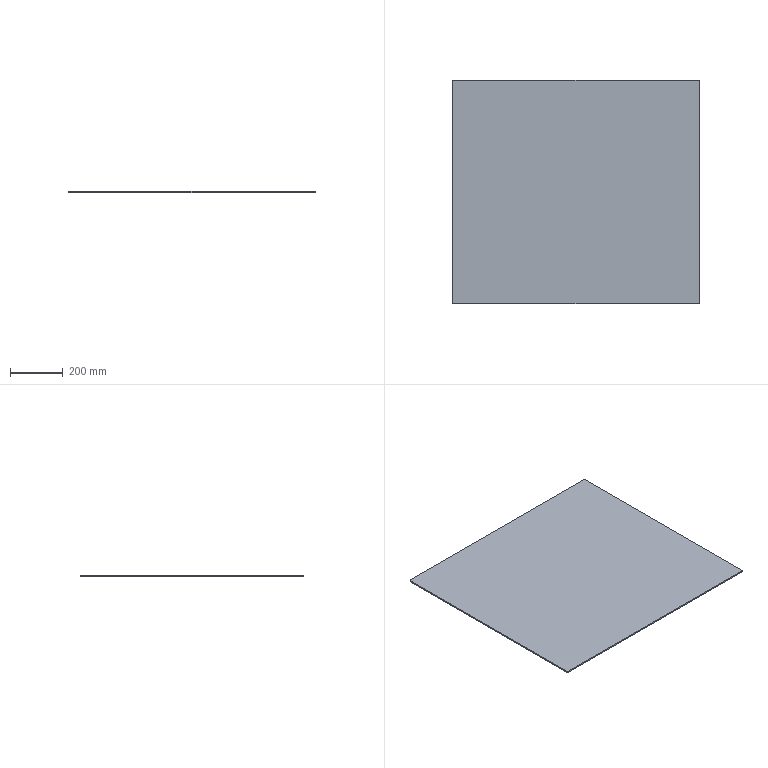Part | STEP file | 001-002-Face Plate-8 | 1 solid | 10 faces | box 940 x 850 x 5 mm | volume 3994893 mm3 | plane 6 | cylinder 4 | commonest cylinder face diameters 10 x4
STEP:
#1=CARTESIAN_POINT('',(0.,0.,0.));
#2=DIRECTION('',(0.,0.,1.));
#3=DIRECTION('',(1.,0.,0.));
#4=AXIS2_PLACEMENT_3D('',#1,#2,#3);
#5=CARTESIAN_POINT('',(470.,-420.,0.));
#6=VERTEX_POINT('',#5);
#7=CARTESIAN_POINT('',(470.,420.,0.));
#8=VERTEX_POINT('',#7);
#9=CARTESIAN_POINT('',(470.,-425.,0.));
#10=DIRECTION('',(0.,1.,0.));
#11=VECTOR('',#10,1.);
#12=LINE('',#9,#11);
#13=CARTESIAN_POINT('',(470.,-425.,5.));
#14=DIRECTION('',(-1.,0.,0.));
#15=DIRECTION('',(0.,0.,1.));
#16=AXIS2_PLACEMENT_3D('',#13,#14,#15);
#17=PLANE('',#16);
#18=CARTESIAN_POINT('',(-5.,0.));
#19=DIRECTION('',(0.,1.));
#20=VECTOR('',#19,1.);
#21=LINE('',#18,#20);
#22=(GEOMETRIC_REPRESENTATION_CONTEXT(2)PARAMETRIC_REPRESENTATION_CONTEXT()REPRESENTATION_CONTEXT('',''));
#23=DEFINITIONAL_REPRESENTATION('',(#21),#22);
#24=PCURVE('',#17,#23);
#25=CARTESIAN_POINT('',(0.,0.,0.));
#26=DIRECTION('',(0.,0.,-1.));
#27=DIRECTION('',(-1.,0.,0.));
#28=AXIS2_PLACEMENT_3D('',#25,#26,#27);
#29=PLANE('',#28);
#30=CARTESIAN_POINT('',(-470.,-425.));
#31=DIRECTION('',(0.,1.));
#32=VECTOR('',#31,1.);
#33=LINE('',#30,#32);
#34=(GEOMETRIC_REPRESENTATION_CONTEXT(2)PARAMETRIC_REPRESENTATION_CONTEXT()REPRESENTATION_CONTEXT('',''));
#35=DEFINITIONAL_REPRESENTATION('',(#33),#34);
#36=PCURVE('',#29,#35);
#37=SURFACE_CURVE('',#12,(#24,#36),.PCURVE_S1.);
#38=EDGE_CURVE('',#6,#8,#37,.T.);
#39=ORIENTED_EDGE('',*,*,#38,.T.);
#40=CARTESIAN_POINT('',(470.,420.,5.));
#41=VERTEX_POINT('',#40);
#42=CARTESIAN_POINT('',(470.,420.,5.));
#43=DIRECTION('',(0.,0.,1.));
#44=VECTOR('',#43,1.);
#45=LINE('',#42,#44);
#46=CARTESIAN_POINT('',(0.,845.));
#47=DIRECTION('',(1.,0.));
#48=VECTOR('',#47,1.);
#49=LINE('',#46,#48);
#50=(GEOMETRIC_REPRESENTATION_CONTEXT(2)PARAMETRIC_REPRESENTATION_CONTEXT()REPRESENTATION_CONTEXT('',''));
#51=DEFINITIONAL_REPRESENTATION('',(#49),#50);
#52=PCURVE('',#17,#51);
#53=CARTESIAN_POINT('',(465.,420.,5.));
#54=DIRECTION('',(0.,0.,-1.));
#55=DIRECTION('',(-1.,0.,0.));
#56=AXIS2_PLACEMENT_3D('',#53,#54,#55);
#57=CYLINDRICAL_SURFACE('',#56,5.);
#58=CARTESIAN_POINT('',(3.142,0.));
#59=DIRECTION('',(0.,-1.));
#60=VECTOR('',#59,1.);
#61=LINE('',#58,#60);
#62=(GEOMETRIC_REPRESENTATION_CONTEXT(2)PARAMETRIC_REPRESENTATION_CONTEXT()REPRESENTATION_CONTEXT('',''));
#63=DEFINITIONAL_REPRESENTATION('',(#61),#62);
#64=PCURVE('',#57,#63);
#65=SURFACE_CURVE('',#45,(#52,#64),.PCURVE_S1.);
#66=EDGE_CURVE('',#8,#41,#65,.T.);
#67=ORIENTED_EDGE('',*,*,#66,.T.);
#68=CARTESIAN_POINT('',(470.,-420.,5.));
#69=VERTEX_POINT('',#68);
#70=CARTESIAN_POINT('',(470.,-425.,5.));
#71=DIRECTION('',(0.,1.,0.));
#72=VECTOR('',#71,1.);
#73=LINE('',#70,#72);
#74=CARTESIAN_POINT('',(0.,0.));
#75=DIRECTION('',(0.,1.));
#76=VECTOR('',#75,1.);
#77=LINE('',#74,#76);
#78=(GEOMETRIC_REPRESENTATION_CONTEXT(2)PARAMETRIC_REPRESENTATION_CONTEXT()REPRESENTATION_CONTEXT('',''));
#79=DEFINITIONAL_REPRESENTATION('',(#77),#78);
#80=PCURVE('',#17,#79);
#81=CARTESIAN_POINT('',(0.,0.,5.));
#82=DIRECTION('',(0.,0.,-1.));
#83=DIRECTION('',(-1.,0.,0.));
#84=AXIS2_PLACEMENT_3D('',#81,#82,#83);
#85=PLANE('',#84);
#86=CARTESIAN_POINT('',(-470.,-425.));
#87=DIRECTION('',(0.,1.));
#88=VECTOR('',#87,1.);
#89=LINE('',#86,#88);
#90=(GEOMETRIC_REPRESENTATION_CONTEXT(2)PARAMETRIC_REPRESENTATION_CONTEXT()REPRESENTATION_CONTEXT('',''));
#91=DEFINITIONAL_REPRESENTATION('',(#89),#90);
#92=PCURVE('',#85,#91);
#93=SURFACE_CURVE('',#73,(#80,#92),.PCURVE_S1.);
#94=EDGE_CURVE('',#69,#41,#93,.T.);
#95=ORIENTED_EDGE('',*,*,#94,.F.);
#96=CARTESIAN_POINT('',(470.,-420.,5.));
#97=DIRECTION('',(0.,0.,-1.));
#98=VECTOR('',#97,1.);
#99=LINE('',#96,#98);
#100=CARTESIAN_POINT('',(0.,5.));
#101=DIRECTION('',(-1.,0.));
#102=VECTOR('',#101,1.);
#103=LINE('',#100,#102);
#104=(GEOMETRIC_REPRESENTATION_CONTEXT(2)PARAMETRIC_REPRESENTATION_CONTEXT()REPRESENTATION_CONTEXT('',''));
#105=DEFINITIONAL_REPRESENTATION('',(#103),#104);
#106=PCURVE('',#17,#105);
#107=CARTESIAN_POINT('',(465.,-420.,5.));
#108=DIRECTION('',(0.,0.,-1.));
#109=DIRECTION('',(-1.,0.,0.));
#110=AXIS2_PLACEMENT_3D('',#107,#108,#109);
#111=CYLINDRICAL_SURFACE('',#110,5.);
#112=CARTESIAN_POINT('',(3.142,0.));
#113=DIRECTION('',(0.,1.));
#114=VECTOR('',#113,1.);
#115=LINE('',#112,#114);
#116=(GEOMETRIC_REPRESENTATION_CONTEXT(2)PARAMETRIC_REPRESENTATION_CONTEXT()REPRESENTATION_CONTEXT('',''));
#117=DEFINITIONAL_REPRESENTATION('',(#115),#116);
#118=PCURVE('',#111,#117);
#119=SURFACE_CURVE('',#99,(#106,#118),.PCURVE_S1.);
#120=EDGE_CURVE('',#69,#6,#119,.T.);
#121=ORIENTED_EDGE('',*,*,#120,.T.);
#122=EDGE_LOOP('',(#39,#67,#95,#121));
#123=FACE_BOUND('',#122,.T.);
#124=ADVANCED_FACE('',(#123),#17,.F.);
#125=CARTESIAN_POINT('',(465.,425.,0.));
#126=VERTEX_POINT('',#125);
#127=CARTESIAN_POINT('',(-465.,425.,0.));
#128=VERTEX_POINT('',#127);
#129=CARTESIAN_POINT('',(-470.,425.,0.));
#130=DIRECTION('',(-1.,0.,0.));
#131=VECTOR('',#130,1.);
#132=LINE('',#129,#131);
#133=CARTESIAN_POINT('',(-470.,425.,5.));
#134=DIRECTION('',(0.,-1.,0.));
#135=DIRECTION('',(0.,0.,-1.));
#136=AXIS2_PLACEMENT_3D('',#133,#134,#135);
#137=PLANE('',#136);
#138=CARTESIAN_POINT('',(5.,0.));
#139=DIRECTION('',(0.,-1.));
#140=VECTOR('',#139,1.);
#141=LINE('',#138,#140);
#142=(GEOMETRIC_REPRESENTATION_CONTEXT(2)PARAMETRIC_REPRESENTATION_CONTEXT()REPRESENTATION_CONTEXT('',''));
#143=DEFINITIONAL_REPRESENTATION('',(#141),#142);
#144=PCURVE('',#137,#143);
#145=CARTESIAN_POINT('',(470.,425.));
#146=DIRECTION('',(1.,0.));
#147=VECTOR('',#146,1.);
#148=LINE('',#145,#147);
#149=(GEOMETRIC_REPRESENTATION_CONTEXT(2)PARAMETRIC_REPRESENTATION_CONTEXT()REPRESENTATION_CONTEXT('',''));
#150=DEFINITIONAL_REPRESENTATION('',(#148),#149);
#151=PCURVE('',#29,#150);
#152=SURFACE_CURVE('',#132,(#144,#151),.PCURVE_S1.);
#153=EDGE_CURVE('',#126,#128,#152,.T.);
#154=ORIENTED_EDGE('',*,*,#153,.T.);
#155=CARTESIAN_POINT('',(-465.,425.,5.));
#156=VERTEX_POINT('',#155);
#157=CARTESIAN_POINT('',(-465.,425.,5.));
#158=DIRECTION('',(0.,0.,1.));
#159=VECTOR('',#158,1.);
#160=LINE('',#157,#159);
#161=CARTESIAN_POINT('',(0.,5.));
#162=DIRECTION('',(-1.,0.));
#163=VECTOR('',#162,1.);
#164=LINE('',#161,#163);
#165=(GEOMETRIC_REPRESENTATION_CONTEXT(2)PARAMETRIC_REPRESENTATION_CONTEXT()REPRESENTATION_CONTEXT('',''));
#166=DEFINITIONAL_REPRESENTATION('',(#164),#165);
#167=PCURVE('',#137,#166);
#168=CARTESIAN_POINT('',(-465.,420.,5.));
#169=DIRECTION('',(0.,0.,-1.));
#170=DIRECTION('',(-1.,0.,0.));
#171=AXIS2_PLACEMENT_3D('',#168,#169,#170);
#172=CYLINDRICAL_SURFACE('',#171,5.);
#173=CARTESIAN_POINT('',(1.571,0.));
#174=DIRECTION('',(0.,-1.));
#175=VECTOR('',#174,1.);
#176=LINE('',#173,#175);
#177=(GEOMETRIC_REPRESENTATION_CONTEXT(2)PARAMETRIC_REPRESENTATION_CONTEXT()REPRESENTATION_CONTEXT('',''));
#178=DEFINITIONAL_REPRESENTATION('',(#176),#177);
#179=PCURVE('',#172,#178);
#180=SURFACE_CURVE('',#160,(#167,#179),.PCURVE_S1.);
#181=EDGE_CURVE('',#128,#156,#180,.T.);
#182=ORIENTED_EDGE('',*,*,#181,.T.);
#183=CARTESIAN_POINT('',(465.,425.,5.));
#184=VERTEX_POINT('',#183);
#185=CARTESIAN_POINT('',(-470.,425.,5.));
#186=DIRECTION('',(-1.,0.,0.));
#187=VECTOR('',#186,1.);
#188=LINE('',#185,#187);
#189=CARTESIAN_POINT('',(0.,0.));
#190=DIRECTION('',(0.,-1.));
#191=VECTOR('',#190,1.);
#192=LINE('',#189,#191);
#193=(GEOMETRIC_REPRESENTATION_CONTEXT(2)PARAMETRIC_REPRESENTATION_CONTEXT()REPRESENTATION_CONTEXT('',''));
#194=DEFINITIONAL_REPRESENTATION('',(#192),#193);
#195=PCURVE('',#137,#194);
#196=CARTESIAN_POINT('',(470.,425.));
#197=DIRECTION('',(1.,0.));
#198=VECTOR('',#197,1.);
#199=LINE('',#196,#198);
#200=(GEOMETRIC_REPRESENTATION_CONTEXT(2)PARAMETRIC_REPRESENTATION_CONTEXT()REPRESENTATION_CONTEXT('',''));
#201=DEFINITIONAL_REPRESENTATION('',(#199),#200);
#202=PCURVE('',#85,#201);
#203=SURFACE_CURVE('',#188,(#195,#202),.PCURVE_S1.);
#204=EDGE_CURVE('',#184,#156,#203,.T.);
#205=ORIENTED_EDGE('',*,*,#204,.F.);
#206=CARTESIAN_POINT('',(465.,425.,5.));
#207=DIRECTION('',(0.,0.,-1.));
#208=VECTOR('',#207,1.);
#209=LINE('',#206,#208);
#210=CARTESIAN_POINT('',(0.,935.));
#211=DIRECTION('',(1.,0.));
#212=VECTOR('',#211,1.);
#213=LINE('',#210,#212);
#214=(GEOMETRIC_REPRESENTATION_CONTEXT(2)PARAMETRIC_REPRESENTATION_CONTEXT()REPRESENTATION_CONTEXT('',''));
#215=DEFINITIONAL_REPRESENTATION('',(#213),#214);
#216=PCURVE('',#137,#215);
#217=CARTESIAN_POINT('',(1.571,0.));
#218=DIRECTION('',(0.,1.));
#219=VECTOR('',#218,1.);
#220=LINE('',#217,#219);
#221=(GEOMETRIC_REPRESENTATION_CONTEXT(2)PARAMETRIC_REPRESENTATION_CONTEXT()REPRESENTATION_CONTEXT('',''));
#222=DEFINITIONAL_REPRESENTATION('',(#220),#221);
#223=PCURVE('',#57,#222);
#224=SURFACE_CURVE('',#209,(#216,#223),.PCURVE_S1.);
#225=EDGE_CURVE('',#184,#126,#224,.T.);
#226=ORIENTED_EDGE('',*,*,#225,.T.);
#227=EDGE_LOOP('',(#154,#182,#205,#226));
#228=FACE_BOUND('',#227,.T.);
#229=ADVANCED_FACE('',(#228),#137,.F.);
#230=CARTESIAN_POINT('',(-470.,420.,0.));
#231=VERTEX_POINT('',#230);
#232=CARTESIAN_POINT('',(-470.,-420.,0.));
#233=VERTEX_POINT('',#232);
#234=CARTESIAN_POINT('',(-470.,-425.,0.));
#235=DIRECTION('',(0.,-1.,0.));
#236=VECTOR('',#235,1.);
#237=LINE('',#234,#236);
#238=CARTESIAN_POINT('',(-470.,-425.,5.));
#239=DIRECTION('',(1.,0.,0.));
#240=DIRECTION('',(0.,0.,-1.));
#241=AXIS2_PLACEMENT_3D('',#238,#239,#240);
#242=PLANE('',#241);
#243=CARTESIAN_POINT('',(5.,0.));
#244=DIRECTION('',(0.,-1.));
#245=VECTOR('',#244,1.);
#246=LINE('',#243,#245);
#247=(GEOMETRIC_REPRESENTATION_CONTEXT(2)PARAMETRIC_REPRESENTATION_CONTEXT()REPRESENTATION_CONTEXT('',''));
#248=DEFINITIONAL_REPRESENTATION('',(#246),#247);
#249=PCURVE('',#242,#248);
#250=CARTESIAN_POINT('',(470.,-425.));
#251=DIRECTION('',(0.,-1.));
#252=VECTOR('',#251,1.);
#253=LINE('',#250,#252);
#254=(GEOMETRIC_REPRESENTATION_CONTEXT(2)PARAMETRIC_REPRESENTATION_CONTEXT()REPRESENTATION_CONTEXT('',''));
#255=DEFINITIONAL_REPRESENTATION('',(#253),#254);
#256=PCURVE('',#29,#255);
#257=SURFACE_CURVE('',#237,(#249,#256),.PCURVE_S1.);
#258=EDGE_CURVE('',#231,#233,#257,.T.);
#259=ORIENTED_EDGE('',*,*,#258,.T.);
#260=CARTESIAN_POINT('',(-470.,-420.,5.));
#261=VERTEX_POINT('',#260);
#262=CARTESIAN_POINT('',(-470.,-420.,5.));
#263=DIRECTION('',(0.,0.,1.));
#264=VECTOR('',#263,1.);
#265=LINE('',#262,#264);
#266=CARTESIAN_POINT('',(0.,5.));
#267=DIRECTION('',(-1.,0.));
#268=VECTOR('',#267,1.);
#269=LINE('',#266,#268);
#270=(GEOMETRIC_REPRESENTATION_CONTEXT(2)PARAMETRIC_REPRESENTATION_CONTEXT()REPRESENTATION_CONTEXT('',''));
#271=DEFINITIONAL_REPRESENTATION('',(#269),#270);
#272=PCURVE('',#242,#271);
#273=CARTESIAN_POINT('',(-465.,-420.,5.));
#274=DIRECTION('',(0.,0.,-1.));
#275=DIRECTION('',(-1.,0.,0.));
#276=AXIS2_PLACEMENT_3D('',#273,#274,#275);
#277=CYLINDRICAL_SURFACE('',#276,5.);
#278=CARTESIAN_POINT('',(6.283,0.));
#279=DIRECTION('',(0.,-1.));
#280=VECTOR('',#279,1.);
#281=LINE('',#278,#280);
#282=(GEOMETRIC_REPRESENTATION_CONTEXT(2)PARAMETRIC_REPRESENTATION_CONTEXT()REPRESENTATION_CONTEXT('',''));
#283=DEFINITIONAL_REPRESENTATION('',(#281),#282);
#284=PCURVE('',#277,#283);
#285=SURFACE_CURVE('',#265,(#272,#284),.PCURVE_S1.);
#286=EDGE_CURVE('',#233,#261,#285,.T.);
#287=ORIENTED_EDGE('',*,*,#286,.T.);
#288=CARTESIAN_POINT('',(-470.,420.,5.));
#289=VERTEX_POINT('',#288);
#290=CARTESIAN_POINT('',(-470.,-425.,5.));
#291=DIRECTION('',(0.,-1.,0.));
#292=VECTOR('',#291,1.);
#293=LINE('',#290,#292);
#294=CARTESIAN_POINT('',(0.,0.));
#295=DIRECTION('',(0.,-1.));
#296=VECTOR('',#295,1.);
#297=LINE('',#294,#296);
#298=(GEOMETRIC_REPRESENTATION_CONTEXT(2)PARAMETRIC_REPRESENTATION_CONTEXT()REPRESENTATION_CONTEXT('',''));
#299=DEFINITIONAL_REPRESENTATION('',(#297),#298);
#300=PCURVE('',#242,#299);
#301=CARTESIAN_POINT('',(470.,-425.));
#302=DIRECTION('',(0.,-1.));
#303=VECTOR('',#302,1.);
#304=LINE('',#301,#303);
#305=(GEOMETRIC_REPRESENTATION_CONTEXT(2)PARAMETRIC_REPRESENTATION_CONTEXT()REPRESENTATION_CONTEXT('',''));
#306=DEFINITIONAL_REPRESENTATION('',(#304),#305);
#307=PCURVE('',#85,#306);
#308=SURFACE_CURVE('',#293,(#300,#307),.PCURVE_S1.);
#309=EDGE_CURVE('',#289,#261,#308,.T.);
#310=ORIENTED_EDGE('',*,*,#309,.F.);
#311=CARTESIAN_POINT('',(-470.,420.,5.));
#312=DIRECTION('',(0.,0.,-1.));
#313=VECTOR('',#312,1.);
#314=LINE('',#311,#313);
#315=CARTESIAN_POINT('',(0.,845.));
#316=DIRECTION('',(1.,0.));
#317=VECTOR('',#316,1.);
#318=LINE('',#315,#317);
#319=(GEOMETRIC_REPRESENTATION_CONTEXT(2)PARAMETRIC_REPRESENTATION_CONTEXT()REPRESENTATION_CONTEXT('',''));
#320=DEFINITIONAL_REPRESENTATION('',(#318),#319);
#321=PCURVE('',#242,#320);
#322=CARTESIAN_POINT('',(0.,0.));
#323=DIRECTION('',(0.,1.));
#324=VECTOR('',#323,1.);
#325=LINE('',#322,#324);
#326=(GEOMETRIC_REPRESENTATION_CONTEXT(2)PARAMETRIC_REPRESENTATION_CONTEXT()REPRESENTATION_CONTEXT('',''));
#327=DEFINITIONAL_REPRESENTATION('',(#325),#326);
#328=PCURVE('',#172,#327);
#329=SURFACE_CURVE('',#314,(#321,#328),.PCURVE_S1.);
#330=EDGE_CURVE('',#289,#231,#329,.T.);
#331=ORIENTED_EDGE('',*,*,#330,.T.);
#332=EDGE_LOOP('',(#259,#287,#310,#331));
#333=FACE_BOUND('',#332,.T.);
#334=ADVANCED_FACE('',(#333),#242,.F.);
#335=CARTESIAN_POINT('',(-465.,-425.,5.));
#336=VERTEX_POINT('',#335);
#337=CARTESIAN_POINT('',(465.,-425.,5.));
#338=VERTEX_POINT('',#337);
#339=CARTESIAN_POINT('',(-470.,-425.,5.));
#340=DIRECTION('',(1.,0.,0.));
#341=VECTOR('',#340,1.);
#342=LINE('',#339,#341);
#343=CARTESIAN_POINT('',(-470.,-425.,5.));
#344=DIRECTION('',(0.,1.,0.));
#345=DIRECTION('',(0.,0.,1.));
#346=AXIS2_PLACEMENT_3D('',#343,#344,#345);
#347=PLANE('',#346);
#348=CARTESIAN_POINT('',(0.,0.));
#349=DIRECTION('',(0.,1.));
#350=VECTOR('',#349,1.);
#351=LINE('',#348,#350);
#352=(GEOMETRIC_REPRESENTATION_CONTEXT(2)PARAMETRIC_REPRESENTATION_CONTEXT()REPRESENTATION_CONTEXT('',''));
#353=DEFINITIONAL_REPRESENTATION('',(#351),#352);
#354=PCURVE('',#347,#353);
#355=CARTESIAN_POINT('',(470.,-425.));
#356=DIRECTION('',(-1.,0.));
#357=VECTOR('',#356,1.);
#358=LINE('',#355,#357);
#359=(GEOMETRIC_REPRESENTATION_CONTEXT(2)PARAMETRIC_REPRESENTATION_CONTEXT()REPRESENTATION_CONTEXT('',''));
#360=DEFINITIONAL_REPRESENTATION('',(#358),#359);
#361=PCURVE('',#85,#360);
#362=SURFACE_CURVE('',#342,(#354,#361),.PCURVE_S1.);
#363=EDGE_CURVE('',#336,#338,#362,.T.);
#364=ORIENTED_EDGE('',*,*,#363,.F.);
#365=CARTESIAN_POINT('',(-465.,-425.,0.));
#366=VERTEX_POINT('',#365);
#367=CARTESIAN_POINT('',(-465.,-425.,5.));
#368=DIRECTION('',(0.,0.,-1.));
#369=VECTOR('',#368,1.);
#370=LINE('',#367,#369);
#371=CARTESIAN_POINT('',(0.,5.));
#372=DIRECTION('',(-1.,0.));
#373=VECTOR('',#372,1.);
#374=LINE('',#371,#373);
#375=(GEOMETRIC_REPRESENTATION_CONTEXT(2)PARAMETRIC_REPRESENTATION_CONTEXT()REPRESENTATION_CONTEXT('',''));
#376=DEFINITIONAL_REPRESENTATION('',(#374),#375);
#377=PCURVE('',#347,#376);
#378=CARTESIAN_POINT('',(4.712,0.));
#379=DIRECTION('',(0.,1.));
#380=VECTOR('',#379,1.);
#381=LINE('',#378,#380);
#382=(GEOMETRIC_REPRESENTATION_CONTEXT(2)PARAMETRIC_REPRESENTATION_CONTEXT()REPRESENTATION_CONTEXT('',''));
#383=DEFINITIONAL_REPRESENTATION('',(#381),#382);
#384=PCURVE('',#277,#383);
#385=SURFACE_CURVE('',#370,(#377,#384),.PCURVE_S1.);
#386=EDGE_CURVE('',#336,#366,#385,.T.);
#387=ORIENTED_EDGE('',*,*,#386,.T.);
#388=CARTESIAN_POINT('',(465.,-425.,0.));
#389=VERTEX_POINT('',#388);
#390=CARTESIAN_POINT('',(-470.,-425.,0.));
#391=DIRECTION('',(1.,0.,0.));
#392=VECTOR('',#391,1.);
#393=LINE('',#390,#392);
#394=CARTESIAN_POINT('',(-5.,0.));
#395=DIRECTION('',(0.,1.));
#396=VECTOR('',#395,1.);
#397=LINE('',#394,#396);
#398=(GEOMETRIC_REPRESENTATION_CONTEXT(2)PARAMETRIC_REPRESENTATION_CONTEXT()REPRESENTATION_CONTEXT('',''));
#399=DEFINITIONAL_REPRESENTATION('',(#397),#398);
#400=PCURVE('',#347,#399);
#401=CARTESIAN_POINT('',(470.,-425.));
#402=DIRECTION('',(-1.,0.));
#403=VECTOR('',#402,1.);
#404=LINE('',#401,#403);
#405=(GEOMETRIC_REPRESENTATION_CONTEXT(2)PARAMETRIC_REPRESENTATION_CONTEXT()REPRESENTATION_CONTEXT('',''));
#406=DEFINITIONAL_REPRESENTATION('',(#404),#405);
#407=PCURVE('',#29,#406);
#408=SURFACE_CURVE('',#393,(#400,#407),.PCURVE_S1.);
#409=EDGE_CURVE('',#366,#389,#408,.T.);
#410=ORIENTED_EDGE('',*,*,#409,.T.);
#411=CARTESIAN_POINT('',(465.,-425.,5.));
#412=DIRECTION('',(0.,0.,1.));
#413=VECTOR('',#412,1.);
#414=LINE('',#411,#413);
#415=CARTESIAN_POINT('',(0.,935.));
#416=DIRECTION('',(1.,0.));
#417=VECTOR('',#416,1.);
#418=LINE('',#415,#417);
#419=(GEOMETRIC_REPRESENTATION_CONTEXT(2)PARAMETRIC_REPRESENTATION_CONTEXT()REPRESENTATION_CONTEXT('',''));
#420=DEFINITIONAL_REPRESENTATION('',(#418),#419);
#421=PCURVE('',#347,#420);
#422=CARTESIAN_POINT('',(4.712,0.));
#423=DIRECTION('',(0.,-1.));
#424=VECTOR('',#423,1.);
#425=LINE('',#422,#424);
#426=(GEOMETRIC_REPRESENTATION_CONTEXT(2)PARAMETRIC_REPRESENTATION_CONTEXT()REPRESENTATION_CONTEXT('',''));
#427=DEFINITIONAL_REPRESENTATION('',(#425),#426);
#428=PCURVE('',#111,#427);
#429=SURFACE_CURVE('',#414,(#421,#428),.PCURVE_S1.);
#430=EDGE_CURVE('',#389,#338,#429,.T.);
#431=ORIENTED_EDGE('',*,*,#430,.T.);
#432=EDGE_LOOP('',(#364,#387,#410,#431));
#433=FACE_BOUND('',#432,.T.);
#434=ADVANCED_FACE('',(#433),#347,.F.);
#435=ORIENTED_EDGE('',*,*,#309,.T.);
#436=CARTESIAN_POINT('',(-465.,-420.,5.));
#437=DIRECTION('',(0.,0.,1.));
#438=DIRECTION('',(-1.,0.,0.));
#439=AXIS2_PLACEMENT_3D('',#436,#437,#438);
#440=CIRCLE('',#439,5.);
#441=CARTESIAN_POINT('',(470.,-420.));
#442=CARTESIAN_POINT('',(470.,-428.66));
#443=CARTESIAN_POINT('',(462.5,-424.33));
#444=CARTESIAN_POINT('',(455.,-420.));
#445=CARTESIAN_POINT('',(462.5,-415.67));
#446=CARTESIAN_POINT('',(470.,-411.34));
#447=CARTESIAN_POINT('',(470.,-420.));
#448=(BOUNDED_CURVE()B_SPLINE_CURVE(2,(#441,#442,#443,#444,#445,#446,#447),.UNSPECIFIED.,.T.,.F.)B_SPLINE_CURVE_WITH_KNOTS((1,2,2,2,2,1),(-2.094,0.,2.094,4.189,6.283,8.378),.UNSPECIFIED.)CURVE()GEOMETRIC_REPRESENTATION_ITEM()RATIONAL_B_SPLINE_CURVE((1.,0.5,1.,0.5,1.,0.5,1.))REPRESENTATION_ITEM(''));
#449=(GEOMETRIC_REPRESENTATION_CONTEXT(2)PARAMETRIC_REPRESENTATION_CONTEXT()REPRESENTATION_CONTEXT('',''));
#450=DEFINITIONAL_REPRESENTATION('',(#448),#449);
#451=PCURVE('',#85,#450);
#452=CARTESIAN_POINT('',(6.283,0.));
#453=DIRECTION('',(-1.,0.));
#454=VECTOR('',#453,1.);
#455=LINE('',#452,#454);
#456=(GEOMETRIC_REPRESENTATION_CONTEXT(2)PARAMETRIC_REPRESENTATION_CONTEXT()REPRESENTATION_CONTEXT('',''));
#457=DEFINITIONAL_REPRESENTATION('',(#455),#456);
#458=PCURVE('',#277,#457);
#459=SURFACE_CURVE('',#440,(#451,#458),.PCURVE_S1.);
#460=EDGE_CURVE('',#261,#336,#459,.T.);
#461=ORIENTED_EDGE('',*,*,#460,.T.);
#462=ORIENTED_EDGE('',*,*,#363,.T.);
#463=CARTESIAN_POINT('',(465.,-420.,5.));
#464=DIRECTION('',(0.,0.,1.));
#465=DIRECTION('',(-1.,0.,0.));
#466=AXIS2_PLACEMENT_3D('',#463,#464,#465);
#467=CIRCLE('',#466,5.);
#468=CARTESIAN_POINT('',(-460.,-420.));
#469=CARTESIAN_POINT('',(-460.,-428.66));
#470=CARTESIAN_POINT('',(-467.5,-424.33));
#471=CARTESIAN_POINT('',(-475.,-420.));
#472=CARTESIAN_POINT('',(-467.5,-415.67));
#473=CARTESIAN_POINT('',(-460.,-411.34));
#474=CARTESIAN_POINT('',(-460.,-420.));
#475=(BOUNDED_CURVE()B_SPLINE_CURVE(2,(#468,#469,#470,#471,#472,#473,#474),.UNSPECIFIED.,.T.,.F.)B_SPLINE_CURVE_WITH_KNOTS((1,2,2,2,2,1),(-2.094,0.,2.094,4.189,6.283,8.378),.UNSPECIFIED.)CURVE()GEOMETRIC_REPRESENTATION_ITEM()RATIONAL_B_SPLINE_CURVE((1.,0.5,1.,0.5,1.,0.5,1.))REPRESENTATION_ITEM(''));
#476=(GEOMETRIC_REPRESENTATION_CONTEXT(2)PARAMETRIC_REPRESENTATION_CONTEXT()REPRESENTATION_CONTEXT('',''));
#477=DEFINITIONAL_REPRESENTATION('',(#475),#476);
#478=PCURVE('',#85,#477);
#479=CARTESIAN_POINT('',(6.283,0.));
#480=DIRECTION('',(-1.,0.));
#481=VECTOR('',#480,1.);
#482=LINE('',#479,#481);
#483=(GEOMETRIC_REPRESENTATION_CONTEXT(2)PARAMETRIC_REPRESENTATION_CONTEXT()REPRESENTATION_CONTEXT('',''));
#484=DEFINITIONAL_REPRESENTATION('',(#482),#483);
#485=PCURVE('',#111,#484);
#486=SURFACE_CURVE('',#467,(#478,#485),.PCURVE_S1.);
#487=EDGE_CURVE('',#338,#69,#486,.T.);
#488=ORIENTED_EDGE('',*,*,#487,.T.);
#489=ORIENTED_EDGE('',*,*,#94,.T.);
#490=CARTESIAN_POINT('',(465.,420.,5.));
#491=DIRECTION('',(0.,0.,1.));
#492=DIRECTION('',(-1.,0.,0.));
#493=AXIS2_PLACEMENT_3D('',#490,#491,#492);
#494=CIRCLE('',#493,5.);
#495=CARTESIAN_POINT('',(-460.,420.));
#496=CARTESIAN_POINT('',(-460.,411.34));
#497=CARTESIAN_POINT('',(-467.5,415.67));
#498=CARTESIAN_POINT('',(-475.,420.));
#499=CARTESIAN_POINT('',(-467.5,424.33));
#500=CARTESIAN_POINT('',(-460.,428.66));
#501=CARTESIAN_POINT('',(-460.,420.));
#502=(BOUNDED_CURVE()B_SPLINE_CURVE(2,(#495,#496,#497,#498,#499,#500,#501),.UNSPECIFIED.,.T.,.F.)B_SPLINE_CURVE_WITH_KNOTS((1,2,2,2,2,1),(-2.094,0.,2.094,4.189,6.283,8.378),.UNSPECIFIED.)CURVE()GEOMETRIC_REPRESENTATION_ITEM()RATIONAL_B_SPLINE_CURVE((1.,0.5,1.,0.5,1.,0.5,1.))REPRESENTATION_ITEM(''));
#503=(GEOMETRIC_REPRESENTATION_CONTEXT(2)PARAMETRIC_REPRESENTATION_CONTEXT()REPRESENTATION_CONTEXT('',''));
#504=DEFINITIONAL_REPRESENTATION('',(#502),#503);
#505=PCURVE('',#85,#504);
#506=CARTESIAN_POINT('',(6.283,0.));
#507=DIRECTION('',(-1.,0.));
#508=VECTOR('',#507,1.);
#509=LINE('',#506,#508);
#510=(GEOMETRIC_REPRESENTATION_CONTEXT(2)PARAMETRIC_REPRESENTATION_CONTEXT()REPRESENTATION_CONTEXT('',''));
#511=DEFINITIONAL_REPRESENTATION('',(#509),#510);
#512=PCURVE('',#57,#511);
#513=SURFACE_CURVE('',#494,(#505,#512),.PCURVE_S1.);
#514=EDGE_CURVE('',#41,#184,#513,.T.);
#515=ORIENTED_EDGE('',*,*,#514,.T.);
#516=ORIENTED_EDGE('',*,*,#204,.T.);
#517=CARTESIAN_POINT('',(-465.,420.,5.));
#518=DIRECTION('',(0.,0.,1.));
#519=DIRECTION('',(-1.,0.,0.));
#520=AXIS2_PLACEMENT_3D('',#517,#518,#519);
#521=CIRCLE('',#520,5.);
#522=CARTESIAN_POINT('',(470.,420.));
#523=CARTESIAN_POINT('',(470.,411.34));
#524=CARTESIAN_POINT('',(462.5,415.67));
#525=CARTESIAN_POINT('',(455.,420.));
#526=CARTESIAN_POINT('',(462.5,424.33));
#527=CARTESIAN_POINT('',(470.,428.66));
#528=CARTESIAN_POINT('',(470.,420.));
#529=(BOUNDED_CURVE()B_SPLINE_CURVE(2,(#522,#523,#524,#525,#526,#527,#528),.UNSPECIFIED.,.T.,.F.)B_SPLINE_CURVE_WITH_KNOTS((1,2,2,2,2,1),(-2.094,0.,2.094,4.189,6.283,8.378),.UNSPECIFIED.)CURVE()GEOMETRIC_REPRESENTATION_ITEM()RATIONAL_B_SPLINE_CURVE((1.,0.5,1.,0.5,1.,0.5,1.))REPRESENTATION_ITEM(''));
#530=(GEOMETRIC_REPRESENTATION_CONTEXT(2)PARAMETRIC_REPRESENTATION_CONTEXT()REPRESENTATION_CONTEXT('',''));
#531=DEFINITIONAL_REPRESENTATION('',(#529),#530);
#532=PCURVE('',#85,#531);
#533=CARTESIAN_POINT('',(6.283,0.));
#534=DIRECTION('',(-1.,0.));
#535=VECTOR('',#534,1.);
#536=LINE('',#533,#535);
#537=(GEOMETRIC_REPRESENTATION_CONTEXT(2)PARAMETRIC_REPRESENTATION_CONTEXT()REPRESENTATION_CONTEXT('',''));
#538=DEFINITIONAL_REPRESENTATION('',(#536),#537);
#539=PCURVE('',#172,#538);
#540=SURFACE_CURVE('',#521,(#532,#539),.PCURVE_S1.);
#541=EDGE_CURVE('',#156,#289,#540,.T.);
#542=ORIENTED_EDGE('',*,*,#541,.T.);
#543=EDGE_LOOP('',(#435,#461,#462,#488,#489,#515,#516,#542));
#544=FACE_BOUND('',#543,.T.);
#545=ADVANCED_FACE('',(#544),#85,.F.);
#546=ORIENTED_EDGE('',*,*,#409,.F.);
#547=CARTESIAN_POINT('',(-465.,-420.,0.));
#548=DIRECTION('',(0.,0.,-1.));
#549=DIRECTION('',(-1.,0.,0.));
#550=AXIS2_PLACEMENT_3D('',#547,#548,#549);
#551=CIRCLE('',#550,5.);
#552=CARTESIAN_POINT('',(465.,-420.));
#553=DIRECTION('',(1.,0.));
#554=AXIS2_PLACEMENT_2D('',#552,#553);
#555=CIRCLE('',#554,5.);
#556=(GEOMETRIC_REPRESENTATION_CONTEXT(2)PARAMETRIC_REPRESENTATION_CONTEXT()REPRESENTATION_CONTEXT('',''));
#557=DEFINITIONAL_REPRESENTATION('',(#555),#556);
#558=PCURVE('',#29,#557);
#559=CARTESIAN_POINT('',(0.,5.));
#560=DIRECTION('',(1.,0.));
#561=VECTOR('',#560,1.);
#562=LINE('',#559,#561);
#563=(GEOMETRIC_REPRESENTATION_CONTEXT(2)PARAMETRIC_REPRESENTATION_CONTEXT()REPRESENTATION_CONTEXT('',''));
#564=DEFINITIONAL_REPRESENTATION('',(#562),#563);
#565=PCURVE('',#277,#564);
#566=SURFACE_CURVE('',#551,(#558,#565),.PCURVE_S1.);
#567=EDGE_CURVE('',#366,#233,#566,.T.);
#568=ORIENTED_EDGE('',*,*,#567,.T.);
#569=ORIENTED_EDGE('',*,*,#258,.F.);
#570=CARTESIAN_POINT('',(-465.,420.,0.));
#571=DIRECTION('',(0.,0.,-1.));
#572=DIRECTION('',(-1.,0.,0.));
#573=AXIS2_PLACEMENT_3D('',#570,#571,#572);
#574=CIRCLE('',#573,5.);
#575=CARTESIAN_POINT('',(465.,420.));
#576=DIRECTION('',(1.,0.));
#577=AXIS2_PLACEMENT_2D('',#575,#576);
#578=CIRCLE('',#577,5.);
#579=(GEOMETRIC_REPRESENTATION_CONTEXT(2)PARAMETRIC_REPRESENTATION_CONTEXT()REPRESENTATION_CONTEXT('',''));
#580=DEFINITIONAL_REPRESENTATION('',(#578),#579);
#581=PCURVE('',#29,#580);
#582=CARTESIAN_POINT('',(0.,5.));
#583=DIRECTION('',(1.,0.));
#584=VECTOR('',#583,1.);
#585=LINE('',#582,#584);
#586=(GEOMETRIC_REPRESENTATION_CONTEXT(2)PARAMETRIC_REPRESENTATION_CONTEXT()REPRESENTATION_CONTEXT('',''));
#587=DEFINITIONAL_REPRESENTATION('',(#585),#586);
#588=PCURVE('',#172,#587);
#589=SURFACE_CURVE('',#574,(#581,#588),.PCURVE_S1.);
#590=EDGE_CURVE('',#231,#128,#589,.T.);
#591=ORIENTED_EDGE('',*,*,#590,.T.);
#592=ORIENTED_EDGE('',*,*,#153,.F.);
#593=CARTESIAN_POINT('',(465.,420.,0.));
#594=DIRECTION('',(0.,0.,-1.));
#595=DIRECTION('',(-1.,0.,0.));
#596=AXIS2_PLACEMENT_3D('',#593,#594,#595);
#597=CIRCLE('',#596,5.);
#598=CARTESIAN_POINT('',(-465.,420.));
#599=DIRECTION('',(1.,0.));
#600=AXIS2_PLACEMENT_2D('',#598,#599);
#601=CIRCLE('',#600,5.);
#602=(GEOMETRIC_REPRESENTATION_CONTEXT(2)PARAMETRIC_REPRESENTATION_CONTEXT()REPRESENTATION_CONTEXT('',''));
#603=DEFINITIONAL_REPRESENTATION('',(#601),#602);
#604=PCURVE('',#29,#603);
#605=CARTESIAN_POINT('',(0.,5.));
#606=DIRECTION('',(1.,0.));
#607=VECTOR('',#606,1.);
#608=LINE('',#605,#607);
#609=(GEOMETRIC_REPRESENTATION_CONTEXT(2)PARAMETRIC_REPRESENTATION_CONTEXT()REPRESENTATION_CONTEXT('',''));
#610=DEFINITIONAL_REPRESENTATION('',(#608),#609);
#611=PCURVE('',#57,#610);
#612=SURFACE_CURVE('',#597,(#604,#611),.PCURVE_S1.);
#613=EDGE_CURVE('',#126,#8,#612,.T.);
#614=ORIENTED_EDGE('',*,*,#613,.T.);
#615=ORIENTED_EDGE('',*,*,#38,.F.);
#616=CARTESIAN_POINT('',(465.,-420.,0.));
#617=DIRECTION('',(0.,0.,-1.));
#618=DIRECTION('',(-1.,0.,0.));
#619=AXIS2_PLACEMENT_3D('',#616,#617,#618);
#620=CIRCLE('',#619,5.);
#621=CARTESIAN_POINT('',(-465.,-420.));
#622=DIRECTION('',(1.,0.));
#623=AXIS2_PLACEMENT_2D('',#621,#622);
#624=CIRCLE('',#623,5.);
#625=(GEOMETRIC_REPRESENTATION_CONTEXT(2)PARAMETRIC_REPRESENTATION_CONTEXT()REPRESENTATION_CONTEXT('',''));
#626=DEFINITIONAL_REPRESENTATION('',(#624),#625);
#627=PCURVE('',#29,#626);
#628=CARTESIAN_POINT('',(0.,5.));
#629=DIRECTION('',(1.,0.));
#630=VECTOR('',#629,1.);
#631=LINE('',#628,#630);
#632=(GEOMETRIC_REPRESENTATION_CONTEXT(2)PARAMETRIC_REPRESENTATION_CONTEXT()REPRESENTATION_CONTEXT('',''));
#633=DEFINITIONAL_REPRESENTATION('',(#631),#632);
#634=PCURVE('',#111,#633);
#635=SURFACE_CURVE('',#620,(#627,#634),.PCURVE_S1.);
#636=EDGE_CURVE('',#6,#389,#635,.T.);
#637=ORIENTED_EDGE('',*,*,#636,.T.);
#638=EDGE_LOOP('',(#546,#568,#569,#591,#592,#614,#615,#637));
#639=FACE_BOUND('',#638,.T.);
#640=ADVANCED_FACE('',(#639),#29,.T.);
#641=ORIENTED_EDGE('',*,*,#460,.F.);
#642=ORIENTED_EDGE('',*,*,#286,.F.);
#643=ORIENTED_EDGE('',*,*,#567,.F.);
#644=ORIENTED_EDGE('',*,*,#386,.F.);
#645=EDGE_LOOP('',(#641,#642,#643,#644));
#646=FACE_BOUND('',#645,.T.);
#647=ADVANCED_FACE('',(#646),#277,.T.);
#648=ORIENTED_EDGE('',*,*,#541,.F.);
#649=ORIENTED_EDGE('',*,*,#181,.F.);
#650=ORIENTED_EDGE('',*,*,#590,.F.);
#651=ORIENTED_EDGE('',*,*,#330,.F.);
#652=EDGE_LOOP('',(#648,#649,#650,#651));
#653=FACE_BOUND('',#652,.T.);
#654=ADVANCED_FACE('',(#653),#172,.T.);
#655=ORIENTED_EDGE('',*,*,#514,.F.);
#656=ORIENTED_EDGE('',*,*,#66,.F.);
#657=ORIENTED_EDGE('',*,*,#613,.F.);
#658=ORIENTED_EDGE('',*,*,#225,.F.);
#659=EDGE_LOOP('',(#655,#656,#657,#658));
#660=FACE_BOUND('',#659,.T.);
#661=ADVANCED_FACE('',(#660),#57,.T.);
#662=ORIENTED_EDGE('',*,*,#487,.F.);
#663=ORIENTED_EDGE('',*,*,#430,.F.);
#664=ORIENTED_EDGE('',*,*,#636,.F.);
#665=ORIENTED_EDGE('',*,*,#120,.F.);
#666=EDGE_LOOP('',(#662,#663,#664,#665));
#667=FACE_BOUND('',#666,.T.);
#668=ADVANCED_FACE('',(#667),#111,.T.);
#669=CLOSED_SHELL('',(#124,#229,#334,#434,#545,#640,#647,#654,#661,#668));
#670=MANIFOLD_SOLID_BREP('',#669);
#671=(LENGTH_UNIT()NAMED_UNIT(*)SI_UNIT(.MILLI.,.METRE.));
#672=UNCERTAINTY_MEASURE_WITH_UNIT(LENGTH_MEASURE(0.0000001),#671,'','');
#673=(NAMED_UNIT(*)PLANE_ANGLE_UNIT()SI_UNIT($,.RADIAN.));
#674=(NAMED_UNIT(*)SI_UNIT($,.STERADIAN.)SOLID_ANGLE_UNIT());
#675=(GEOMETRIC_REPRESENTATION_CONTEXT(3)GLOBAL_UNCERTAINTY_ASSIGNED_CONTEXT((#672))GLOBAL_UNIT_ASSIGNED_CONTEXT((#671,#673,#674))REPRESENTATION_CONTEXT('',''));
#676=ADVANCED_BREP_SHAPE_REPRESENTATION('',(#4,#670),#675);